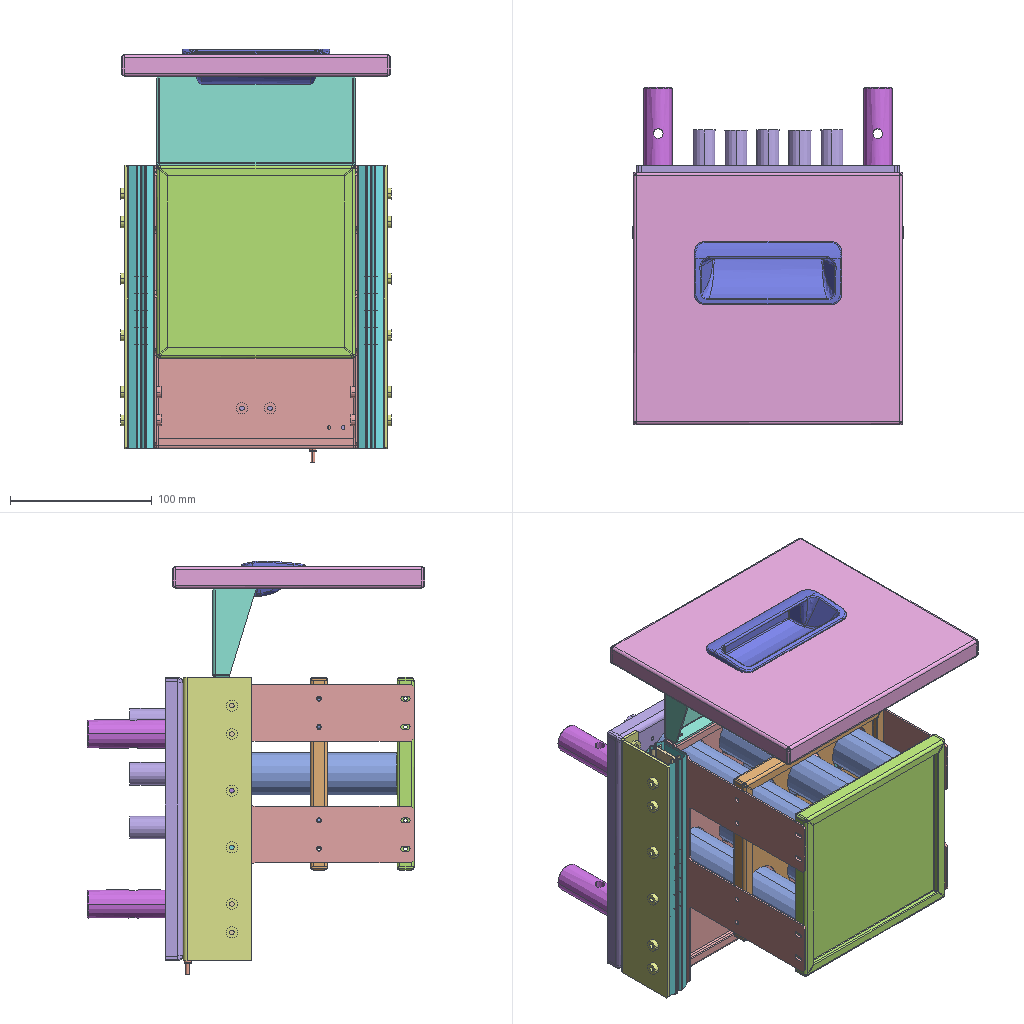Assembly | SolidWorks | 18 different items | 34 placed | box 191 x 238 x 292 mm
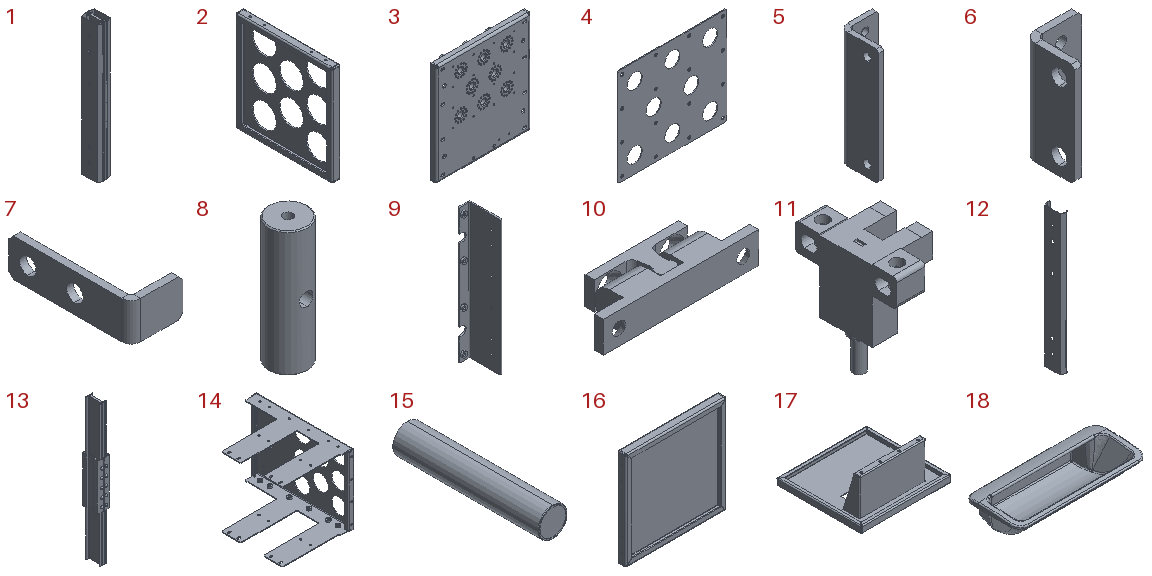Parts list (item | name | quantity | parent item | size | volume | features):
1 | (subassembly) | x2 | - | 19.1 x 27 x 200 mm | 23811 mm3 | features AEMSimFeature 1
2 | - | x1 | - | 12 x 136 x 140 mm | 29958 mm3 | features SMWeldBead 4, EdgeFlange 2, FlatPattern 1, HoleWzd 1, ICE 1, LPattern 1, SMBaseFlange 1, SheetMetal 1
3 | - | x1 | - | 185 x 37.5 x 200 mm | 128218 mm3 | features HoleWzd 6, SMWeldBead 4, LPattern 3, ICE 2, CirPattern 1, Cut 1, EdgeFlange 1, FlatPattern 1, MirrorPattern 1, SMBaseFlange 1, SheetMetal 1
4 | - | x1 | - | 130 x 1 x 116 mm | 12882 mm3 | features LPattern 2, Chamfer 1, Extrusion 1, HoleWzd 1, ICE 1
5 | - | x1 | - | 15 x 17 x 50 mm | 2820 mm3 | features HoleWzd 2, Chamfer 1, FlatPattern 1, SMBaseFlange 1, SheetMetal 1
6 | - | x1 | - | 15 x 15 x 30 mm | 1514 mm3 | features HoleWzd 2, Chamfer 1, FlatPattern 1, SMBaseFlange 1, SheetMetal 1
7 | - | x1 | - | 11 x 26 x 8 mm | 387.699 mm3 | features Chamfer 1, FlatPattern 1, HoleWzd 1, SMBaseFlange 1, SheetMetal 1
8 | - | x4 | - | 20 x 20 x 65 mm | 19038 mm3 | features HoleWzd 2, Chamfer 1, Extrusion 1, ICE 1
9 | - | x2 | - | 20 x 48 x 200 mm | 25515 mm3 | features HoleWzd 2, ICE 2, Chamfer 1, Cut 1, EdgeFlange 1, FlatPattern 1, LPattern 1, SMBaseFlange 1, SheetMetal 1
10 | - | x1 | - | 50 x 15.9 x 10 mm | 4373 mm3 | features BaseBody 2
11 | - | x1 | - | 15.65 x 26 x 28.5 mm | 2575 mm3 | features BaseBody 3, ICE 1
12 | - | x4 | in 1 | 9 x 27 x 200 mm | 4310 mm3 | features BaseBody 1
13 | - | x2 | in 1 | 17.1 x 26 x 200 mm | 15191 mm3 | features BaseBody 3
14 | - | x1 | - | 142 x 200 x 143 mm | 82962 mm3 | features ICE 6, HoleWzd 5, SMWeldBead 4, EdgeFlange 2, Chamfer 1, Fillet 1, FlatPattern 1, MirrorPattern 1, SMBaseFlange 1, SheetMetal 1
15 | - | x8 | - | 30 x 150 x 30 mm | 21279 mm3 | features Chamfer 1, Extrusion 1, RevCut 1
16 | - | x1 | - | 140 x 12 x 136 mm | 40853 mm3 | features SMWeldBead 4, EdgeFlange 2, FlatPattern 1, HoleWzd 1, LPattern 1, MirrorPattern 1, SMBaseFlange 1, SheetMetal 1
17 | - | x1 | - | 190 x 178 x 78 mm | 87665 mm3 | features SMWeldBead 6, EdgeFlange 3, FlatPattern 2, HoleWzd 2, SMBaseFlange 2, SheetMetal 2, Chamfer 1, ICE 1
18 | - | x1 | - | 104 x 48 x 25 mm | 19338 mm3 | features BaseBody 1
Mates (type | each side: item.copy, entity, surface, feature):
In the top assembly
Coincident | 15.1 face plane Boss-Extrude1 | 16.1 face plane Base-Flange1
Concentric | 15.1 face cylinder Boss-Extrude1 | 2.1 face cylinder Cut-Extrude2
Width | 3.1 face plane Edge-Flange1 | 3.1 face plane Edge-Flange1 | 14.1 face plane Edge-Flange1 | 14.1 face plane Edge-Flange1 | 2 times
Coincident | 3.1 face plane Base-Flange1 | 4.1 face plane Boss-Extrude1
Concentric | 3.1 face cylinder Boss-Extrude1 | 4.1 face cylinder Cut-Extrude1
Parallel | 3.1 face plane Edge-Flange1 | 4.1 face plane Boss-Extrude1
Coincident | 3.1 face plane Base-Flange1 | 8.1 face plane Boss-Extrude1
Concentric | 8.1 face cylinder Boss-Extrude1 | 3.1 face cylinder Ø7.0 (7) Diameter Hole1
Coincident | 3.1 face plane Base-Flange1 | 8.2 face plane Boss-Extrude1
Concentric | 8.2 face cylinder Boss-Extrude1 | 3.1 face cylinder Ø7.0 (7) Diameter Hole1
Coincident | 3.1 face plane Base-Flange1 | 8.3 face plane Boss-Extrude1
Concentric | 8.3 face cylinder Boss-Extrude1 | 3.1 face cylinder Ø7.0 (7) Diameter Hole1
Coincident | 3.1 face plane Base-Flange1 | 8.4 face plane Boss-Extrude1
Concentric | 8.4 face cylinder Boss-Extrude1 | 3.1 face cylinder Ø7.0 (7) Diameter Hole1
DistanceDim | 14.1 face plane Base-Flange1 | 3.1 face plane Base-Flange1
Coincident | 3.1 face plane Edge-Flange1 | 9.1 face plane Base-Flange1
Coincident | 3.1 face plane Base-Flange1 | 9.1 face plane Base-Flange1
Coincident | 3.1 face plane Edge-Flange1 | 9.2 face plane Edge-Flange2
Coincident | 3.1 face plane Base-Flange1 | 9.2 face plane Base-Flange1
Coincident | 14.1 face plane Edge-Flange1 | 17.1 face plane Edge-Flange2
Coincident | 14.1 face plane Base-Flange1 | 17.1 face plane Base-Flange2
Width | 14.1 face plane Edge-Flange1 | 14.1 face plane Edge-Flange1 | 16.1 face plane Edge-Flange1 | 16.1 face plane Edge-Flange1
Width | 2.1 face plane Edge-Flange1 | 2.1 face plane Edge-Flange1 | 14.1 face plane Edge-Flange1 | 14.1 face plane Edge-Flange1
Coincident | 14.1 face plane Edge-Flange1 | 12.1 face plane Input 1 | 2 times
Coincident | 14.1 face plane Base-Flange1 | 12.1 face plane Input 1
Coincident | 14.1 face plane Edge-Flange1 | 12.2 face plane Input 1
Coincident | 14.1 face plane Base-Flange1 | 12.2 face plane Input 1
Width | 17.1 face plane Base-Flange2 | 17.1 face plane Base-Flange2 | 14.1 face plane Edge-Flange1 | 14.1 face plane Edge-Flange1
Coincident | 14.1 face plane Edge-Flange1 | 2.1 face plane Edge-Flange1
Coincident | 16.1 face plane Edge-Flange1 | 2.1 face plane Edge-Flange1
Coincident | 14.1 face plane Edge-Flange1 | 16.1 face plane Edge-Flange2
Concentric | 14.1 face cylinder Ø3.5 (3.5) Diameter Hole1 | 2.1 face cylinder M3 Tapped Hole1 | 2 times
Coincident | 9.1 face plane Edge-Flange2 | 12.3 face plane Input 1 | 2 times
Coincident | 12.4 face plane Input 1 | 9.2 face plane Edge-Flange2 | 2 times
Width | 18.1 face plane Input 1 | 18.1 face plane Input 1 | 17.1 face plane Cut-Extrude1 | 17.1 face plane Cut-Extrude1
Width | 17.1 face plane Cut-Extrude1 | 17.1 face plane Cut-Extrude1 | 18.1 face plane Input 1 | 18.1 face plane Input 1
Coincident | 17.1 face plane Base-Flange1 | 18.1 face plane Input 1
Concentric | 6.1 face cylinder M4 Tapped Hole1 | 10.1 face cone 2-1-solid1 | 2 times
Coincident | 6.1 face plane Base-Flange1 | 10.1 face plane 2-1-solid1
Coincident | 3.1 face plane Base-Flange1 | 11.1 face plane Input 3
Concentric | 3.1 face cylinder M3 Tapped Hole2 | 11.1 face cylinder Input 3 | 2 times
Coincident | 14.1 face plane Base-Flange1 | 7.1 face plane Base-Flange1
Concentric | 14.1 face cylinder M3 Tapped Hole1 | 7.1 face cylinder Ø3.5 (3.5) Diameter Hole1 | 2 times
Coincident | 3.1 face plane Base-Flange1 | 5.1 face plane Base-Flange1
Concentric | 3.1 face cylinder Ø4.5 (4.5) Diameter Hole1 | 5.1 face cylinder M4 Tapped Hole3 | 2 times
Concentric | 5.1 face cylinder M4 Tapped Hole2 | 10.1 face cone 1-1-solid1 | 2 times
Coincident | 5.1 face plane Base-Flange1 | 10.1 face plane 1-1-solid1
In subassembly 1
Width | 12.5 face plane Input 1 | 12.5 face plane Input 1 | 13.1 face plane 3-1-solid1 | 13.1 face plane 3-1-solid1
DistanceDim | 13.1 face plane 1-1-solid1 | 12.5 face plane Input 1
DistanceDim | 13.1 face plane 1-1-solid1 | 12.6 face plane Input 1
Width | 13.1 face plane 5-1-solid1 | 13.1 face plane 5-1-solid1 | 12.6 face plane Input 1 | 12.6 face plane Input 1
LimitDistanceDim | 13.1 face plane 1-1-solid1 | 12.5 face plane Input 1
LimitDistanceDim | 13.1 face plane 1-1-solid1 | 12.6 face plane Input 1